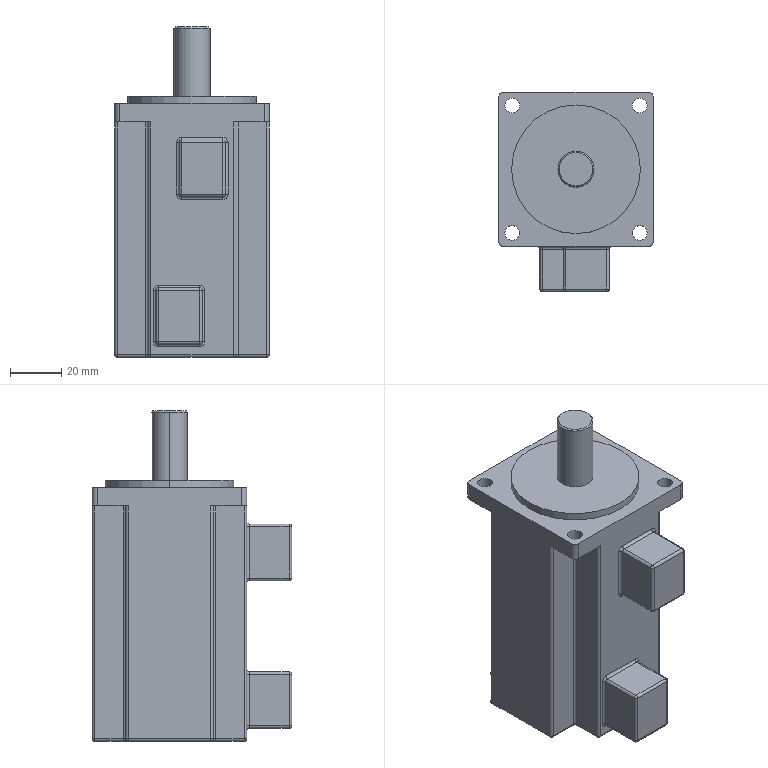Part | SolidWorks | features BaseBody 1 | 1 solid | 124 faces | box 60 x 77.5 x 128.4 mm | volume 315434 mm3 | cylinder 64 | plane 30 | sphere 16 | torus 12 | cone 2 | commonest cylinder face diameters 2 x48 5.8 x8 4 x4 14 x2 50 x2